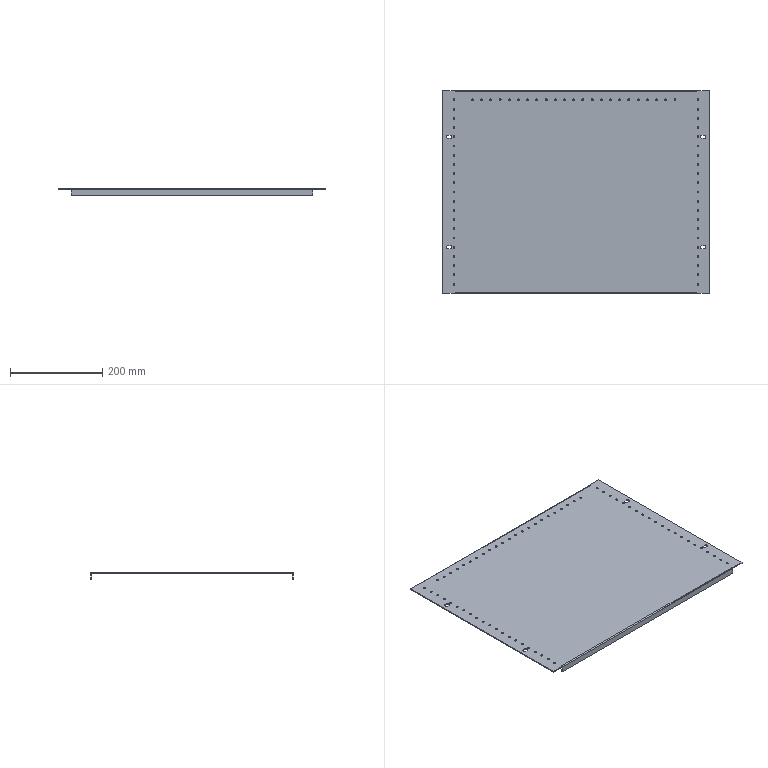Part | SolidWorks | features ICE 4, MoveFace 2, BaseBody 1 | 1 solid | 180 faces | box 580 x 440 x 15 mm | volume 534266 mm3 | cylinder 146 | plane 34 | commonest cylinder face diameters 4.2 x132 7 x12 0.2 x2